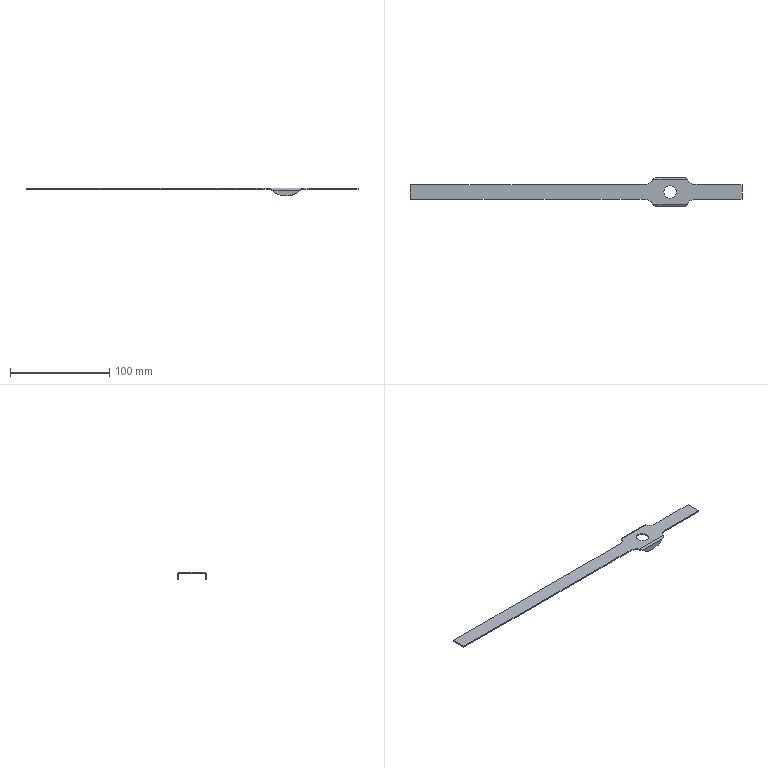Part | STEP file | gslz 2016.10.28-13_id974_x_t | 1 solid | 32 faces | box 335 x 29 x 8 mm | volume 7097 mm3 | other 12 | plane 11 | cylinder 5 | spline 4 | commonest cylinder face diameters 1.5 x2 4 x2 12.3 x1